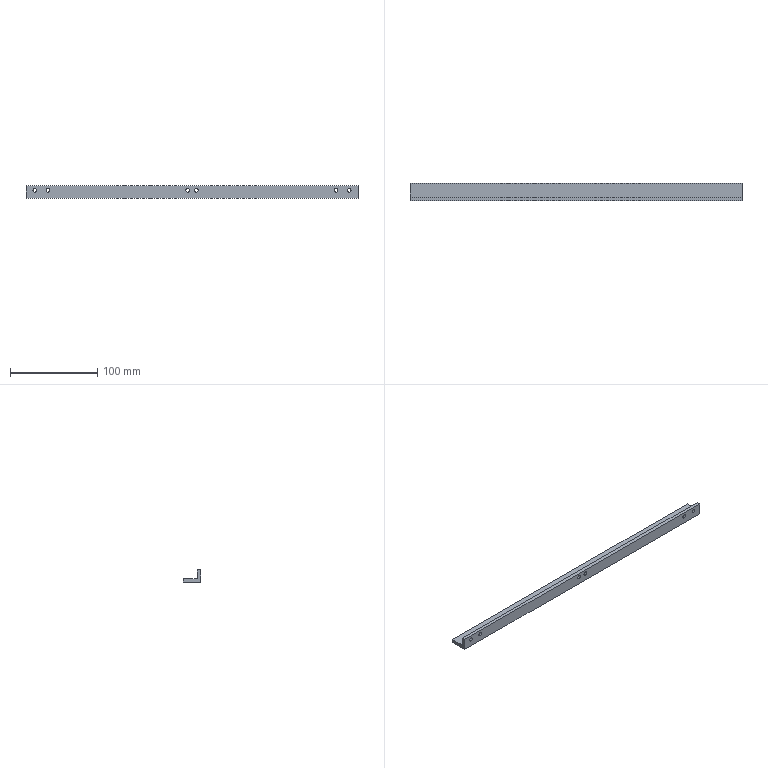Part | SolidWorks | features Extrusion 1, ICE 1 | 1 solid | 20 faces | box 380 x 20 x 14 mm | volume 45267 mm3 | cylinder 12 | plane 8 | commonest cylinder face diameters 4.2 x12
STEP:
#1=CARTESIAN_POINT('',(-5.,4.,-2.1));
#2=VERTEX_POINT('',#1);
#3=CARTESIAN_POINT('',(-5.,4.,2.1));
#4=VERTEX_POINT('',#3);
#5=CARTESIAN_POINT('',(-5.,4.,0.));
#6=DIRECTION('',(0.,1.,0.));
#7=DIRECTION('',(0.,0.,1.));
#8=AXIS2_PLACEMENT_3D('',#5,#6,#7);
#9=CIRCLE('',#8,2.1);
#10=EDGE_CURVE('',#2,#4,#9,.T.);
#11=ORIENTED_EDGE('',*,*,#10,.T.);
#12=CARTESIAN_POINT('',(-5.,0.,2.1));
#13=VERTEX_POINT('',#12);
#14=CARTESIAN_POINT('',(-5.,4.,2.1));
#15=DIRECTION('',(0.,-1.,0.));
#16=VECTOR('',#15,1000.);
#17=LINE('',#14,#16);
#18=EDGE_CURVE('',#4,#13,#17,.T.);
#19=ORIENTED_EDGE('',*,*,#18,.T.);
#20=CARTESIAN_POINT('',(-5.,0.,-2.1));
#21=VERTEX_POINT('',#20);
#22=CARTESIAN_POINT('',(-5.,0.,0.));
#23=DIRECTION('',(0.,1.,0.));
#24=DIRECTION('',(0.,0.,1.));
#25=AXIS2_PLACEMENT_3D('',#22,#23,#24);
#26=CIRCLE('',#25,2.1);
#27=EDGE_CURVE('',#21,#13,#26,.T.);
#28=ORIENTED_EDGE('',*,*,#27,.F.);
#29=CARTESIAN_POINT('',(-5.,4.,-2.1));
#30=DIRECTION('',(0.,-1.,0.));
#31=VECTOR('',#30,1000.);
#32=LINE('',#29,#31);
#33=EDGE_CURVE('',#2,#21,#32,.T.);
#34=ORIENTED_EDGE('',*,*,#33,.F.);
#35=EDGE_LOOP('',(#11,#19,#28,#34));
#36=FACE_OUTER_BOUND('',#35,.T.);
#37=CARTESIAN_POINT('',(-5.,4.,0.));
#38=DIRECTION('',(0.,-1.,0.));
#39=DIRECTION('',(0.,0.,-1.));
#40=AXIS2_PLACEMENT_3D('',#37,#38,#39);
#41=CYLINDRICAL_SURFACE('',#40,2.1);
#42=ADVANCED_FACE('',(#36),#41,.F.);
#43=CARTESIAN_POINT('',(5.,4.,-2.1));
#44=VERTEX_POINT('',#43);
#45=CARTESIAN_POINT('',(5.,4.,2.1));
#46=VERTEX_POINT('',#45);
#47=CARTESIAN_POINT('',(5.,4.,0.));
#48=DIRECTION('',(0.,1.,0.));
#49=DIRECTION('',(0.,0.,1.));
#50=AXIS2_PLACEMENT_3D('',#47,#48,#49);
#51=CIRCLE('',#50,2.1);
#52=EDGE_CURVE('',#44,#46,#51,.T.);
#53=ORIENTED_EDGE('',*,*,#52,.T.);
#54=CARTESIAN_POINT('',(5.,0.,2.1));
#55=VERTEX_POINT('',#54);
#56=CARTESIAN_POINT('',(5.,4.,2.1));
#57=DIRECTION('',(0.,-1.,0.));
#58=VECTOR('',#57,1000.);
#59=LINE('',#56,#58);
#60=EDGE_CURVE('',#46,#55,#59,.T.);
#61=ORIENTED_EDGE('',*,*,#60,.T.);
#62=CARTESIAN_POINT('',(5.,0.,-2.1));
#63=VERTEX_POINT('',#62);
#64=CARTESIAN_POINT('',(5.,0.,0.));
#65=DIRECTION('',(0.,1.,0.));
#66=DIRECTION('',(0.,0.,1.));
#67=AXIS2_PLACEMENT_3D('',#64,#65,#66);
#68=CIRCLE('',#67,2.1);
#69=EDGE_CURVE('',#63,#55,#68,.T.);
#70=ORIENTED_EDGE('',*,*,#69,.F.);
#71=CARTESIAN_POINT('',(5.,4.,-2.1));
#72=DIRECTION('',(0.,-1.,0.));
#73=VECTOR('',#72,1000.);
#74=LINE('',#71,#73);
#75=EDGE_CURVE('',#44,#63,#74,.T.);
#76=ORIENTED_EDGE('',*,*,#75,.F.);
#77=EDGE_LOOP('',(#53,#61,#70,#76));
#78=FACE_OUTER_BOUND('',#77,.T.);
#79=CARTESIAN_POINT('',(5.,4.,0.));
#80=DIRECTION('',(0.,-1.,0.));
#81=DIRECTION('',(0.,0.,-1.));
#82=AXIS2_PLACEMENT_3D('',#79,#80,#81);
#83=CYLINDRICAL_SURFACE('',#82,2.1);
#84=ADVANCED_FACE('',(#78),#83,.F.);
#85=CARTESIAN_POINT('',(180.,4.,-2.1));
#86=VERTEX_POINT('',#85);
#87=CARTESIAN_POINT('',(180.,4.,2.1));
#88=VERTEX_POINT('',#87);
#89=CARTESIAN_POINT('',(180.,4.,0.));
#90=DIRECTION('',(0.,1.,0.));
#91=DIRECTION('',(0.,0.,-1.));
#92=AXIS2_PLACEMENT_3D('',#89,#90,#91);
#93=CIRCLE('',#92,2.1);
#94=EDGE_CURVE('',#86,#88,#93,.T.);
#95=ORIENTED_EDGE('',*,*,#94,.T.);
#96=CARTESIAN_POINT('',(180.,0.,2.1));
#97=VERTEX_POINT('',#96);
#98=CARTESIAN_POINT('',(180.,4.,2.1));
#99=DIRECTION('',(0.,-1.,0.));
#100=VECTOR('',#99,1000.);
#101=LINE('',#98,#100);
#102=EDGE_CURVE('',#88,#97,#101,.T.);
#103=ORIENTED_EDGE('',*,*,#102,.T.);
#104=CARTESIAN_POINT('',(180.,0.,-2.1));
#105=VERTEX_POINT('',#104);
#106=CARTESIAN_POINT('',(180.,0.,0.));
#107=DIRECTION('',(0.,1.,0.));
#108=DIRECTION('',(0.,0.,-1.));
#109=AXIS2_PLACEMENT_3D('',#106,#107,#108);
#110=CIRCLE('',#109,2.1);
#111=EDGE_CURVE('',#105,#97,#110,.T.);
#112=ORIENTED_EDGE('',*,*,#111,.F.);
#113=CARTESIAN_POINT('',(180.,4.,-2.1));
#114=DIRECTION('',(0.,-1.,0.));
#115=VECTOR('',#114,1000.);
#116=LINE('',#113,#115);
#117=EDGE_CURVE('',#86,#105,#116,.T.);
#118=ORIENTED_EDGE('',*,*,#117,.F.);
#119=EDGE_LOOP('',(#95,#103,#112,#118));
#120=FACE_OUTER_BOUND('',#119,.T.);
#121=CARTESIAN_POINT('',(180.,4.,0.));
#122=DIRECTION('',(0.,-1.,0.));
#123=DIRECTION('',(0.,0.,-1.));
#124=AXIS2_PLACEMENT_3D('',#121,#122,#123);
#125=CYLINDRICAL_SURFACE('',#124,2.1);
#126=ADVANCED_FACE('',(#120),#125,.F.);
#127=CARTESIAN_POINT('',(165.,4.,-2.1));
#128=VERTEX_POINT('',#127);
#129=CARTESIAN_POINT('',(165.,4.,2.1));
#130=VERTEX_POINT('',#129);
#131=CARTESIAN_POINT('',(165.,4.,0.));
#132=DIRECTION('',(0.,1.,0.));
#133=DIRECTION('',(0.,0.,-1.));
#134=AXIS2_PLACEMENT_3D('',#131,#132,#133);
#135=CIRCLE('',#134,2.1);
#136=EDGE_CURVE('',#128,#130,#135,.T.);
#137=ORIENTED_EDGE('',*,*,#136,.T.);
#138=CARTESIAN_POINT('',(165.,0.,2.1));
#139=VERTEX_POINT('',#138);
#140=CARTESIAN_POINT('',(165.,4.,2.1));
#141=DIRECTION('',(0.,-1.,0.));
#142=VECTOR('',#141,1000.);
#143=LINE('',#140,#142);
#144=EDGE_CURVE('',#130,#139,#143,.T.);
#145=ORIENTED_EDGE('',*,*,#144,.T.);
#146=CARTESIAN_POINT('',(165.,0.,-2.1));
#147=VERTEX_POINT('',#146);
#148=CARTESIAN_POINT('',(165.,0.,0.));
#149=DIRECTION('',(0.,1.,0.));
#150=DIRECTION('',(0.,0.,-1.));
#151=AXIS2_PLACEMENT_3D('',#148,#149,#150);
#152=CIRCLE('',#151,2.1);
#153=EDGE_CURVE('',#147,#139,#152,.T.);
#154=ORIENTED_EDGE('',*,*,#153,.F.);
#155=CARTESIAN_POINT('',(165.,4.,-2.1));
#156=DIRECTION('',(0.,-1.,0.));
#157=VECTOR('',#156,1000.);
#158=LINE('',#155,#157);
#159=EDGE_CURVE('',#128,#147,#158,.T.);
#160=ORIENTED_EDGE('',*,*,#159,.F.);
#161=EDGE_LOOP('',(#137,#145,#154,#160));
#162=FACE_OUTER_BOUND('',#161,.T.);
#163=CARTESIAN_POINT('',(165.,4.,0.));
#164=DIRECTION('',(0.,-1.,0.));
#165=DIRECTION('',(0.,0.,-1.));
#166=AXIS2_PLACEMENT_3D('',#163,#164,#165);
#167=CYLINDRICAL_SURFACE('',#166,2.1);
#168=ADVANCED_FACE('',(#162),#167,.F.);
#169=CARTESIAN_POINT('',(-165.,4.,-2.1));
#170=VERTEX_POINT('',#169);
#171=CARTESIAN_POINT('',(-165.,4.,2.1));
#172=VERTEX_POINT('',#171);
#173=CARTESIAN_POINT('',(-165.,4.,0.));
#174=DIRECTION('',(0.,1.,0.));
#175=DIRECTION('',(0.,0.,1.));
#176=AXIS2_PLACEMENT_3D('',#173,#174,#175);
#177=CIRCLE('',#176,2.1);
#178=EDGE_CURVE('',#170,#172,#177,.T.);
#179=ORIENTED_EDGE('',*,*,#178,.T.);
#180=CARTESIAN_POINT('',(-165.,0.,2.1));
#181=VERTEX_POINT('',#180);
#182=CARTESIAN_POINT('',(-165.,4.,2.1));
#183=DIRECTION('',(0.,-1.,0.));
#184=VECTOR('',#183,1000.);
#185=LINE('',#182,#184);
#186=EDGE_CURVE('',#172,#181,#185,.T.);
#187=ORIENTED_EDGE('',*,*,#186,.T.);
#188=CARTESIAN_POINT('',(-165.,0.,-2.1));
#189=VERTEX_POINT('',#188);
#190=CARTESIAN_POINT('',(-165.,0.,0.));
#191=DIRECTION('',(0.,1.,0.));
#192=DIRECTION('',(0.,0.,1.));
#193=AXIS2_PLACEMENT_3D('',#190,#191,#192);
#194=CIRCLE('',#193,2.1);
#195=EDGE_CURVE('',#189,#181,#194,.T.);
#196=ORIENTED_EDGE('',*,*,#195,.F.);
#197=CARTESIAN_POINT('',(-165.,4.,-2.1));
#198=DIRECTION('',(0.,-1.,0.));
#199=VECTOR('',#198,1000.);
#200=LINE('',#197,#199);
#201=EDGE_CURVE('',#170,#189,#200,.T.);
#202=ORIENTED_EDGE('',*,*,#201,.F.);
#203=EDGE_LOOP('',(#179,#187,#196,#202));
#204=FACE_OUTER_BOUND('',#203,.T.);
#205=CARTESIAN_POINT('',(-165.,4.,0.));
#206=DIRECTION('',(0.,-1.,0.));
#207=DIRECTION('',(0.,0.,-1.));
#208=AXIS2_PLACEMENT_3D('',#205,#206,#207);
#209=CYLINDRICAL_SURFACE('',#208,2.1);
#210=ADVANCED_FACE('',(#204),#209,.F.);
#211=CARTESIAN_POINT('',(-180.,4.,-2.1));
#212=VERTEX_POINT('',#211);
#213=CARTESIAN_POINT('',(-180.,4.,2.1));
#214=VERTEX_POINT('',#213);
#215=CARTESIAN_POINT('',(-180.,4.,0.));
#216=DIRECTION('',(0.,1.,0.));
#217=DIRECTION('',(0.,0.,1.));
#218=AXIS2_PLACEMENT_3D('',#215,#216,#217);
#219=CIRCLE('',#218,2.1);
#220=EDGE_CURVE('',#212,#214,#219,.T.);
#221=ORIENTED_EDGE('',*,*,#220,.T.);
#222=CARTESIAN_POINT('',(-180.,0.,2.1));
#223=VERTEX_POINT('',#222);
#224=CARTESIAN_POINT('',(-180.,4.,2.1));
#225=DIRECTION('',(0.,-1.,0.));
#226=VECTOR('',#225,1000.);
#227=LINE('',#224,#226);
#228=EDGE_CURVE('',#214,#223,#227,.T.);
#229=ORIENTED_EDGE('',*,*,#228,.T.);
#230=CARTESIAN_POINT('',(-180.,0.,-2.1));
#231=VERTEX_POINT('',#230);
#232=CARTESIAN_POINT('',(-180.,0.,0.));
#233=DIRECTION('',(0.,1.,0.));
#234=DIRECTION('',(0.,0.,1.));
#235=AXIS2_PLACEMENT_3D('',#232,#233,#234);
#236=CIRCLE('',#235,2.1);
#237=EDGE_CURVE('',#231,#223,#236,.T.);
#238=ORIENTED_EDGE('',*,*,#237,.F.);
#239=CARTESIAN_POINT('',(-180.,4.,-2.1));
#240=DIRECTION('',(0.,-1.,0.));
#241=VECTOR('',#240,1000.);
#242=LINE('',#239,#241);
#243=EDGE_CURVE('',#212,#231,#242,.T.);
#244=ORIENTED_EDGE('',*,*,#243,.F.);
#245=EDGE_LOOP('',(#221,#229,#238,#244));
#246=FACE_OUTER_BOUND('',#245,.T.);
#247=CARTESIAN_POINT('',(-180.,4.,0.));
#248=DIRECTION('',(0.,-1.,0.));
#249=DIRECTION('',(0.,0.,-1.));
#250=AXIS2_PLACEMENT_3D('',#247,#248,#249);
#251=CYLINDRICAL_SURFACE('',#250,2.1);
#252=ADVANCED_FACE('',(#246),#251,.F.);
#253=CARTESIAN_POINT('',(190.,4.,5.));
#254=VERTEX_POINT('',#253);
#255=CARTESIAN_POINT('',(190.,4.,-5.));
#256=VERTEX_POINT('',#255);
#257=CARTESIAN_POINT('',(190.,4.,5.));
#258=DIRECTION('',(0.,0.,-1.));
#259=VECTOR('',#258,1000.);
#260=LINE('',#257,#259);
#261=EDGE_CURVE('',#254,#256,#260,.T.);
#262=ORIENTED_EDGE('',*,*,#261,.T.);
#263=CARTESIAN_POINT('',(-190.,4.,-5.));
#264=VERTEX_POINT('',#263);
#265=CARTESIAN_POINT('',(-190.,4.,-5.));
#266=DIRECTION('',(-1.,0.,0.));
#267=VECTOR('',#266,1000.);
#268=LINE('',#265,#267);
#269=EDGE_CURVE('',#256,#264,#268,.T.);
#270=ORIENTED_EDGE('',*,*,#269,.T.);
#271=CARTESIAN_POINT('',(-190.,4.,5.));
#272=VERTEX_POINT('',#271);
#273=CARTESIAN_POINT('',(-190.,4.,5.));
#274=DIRECTION('',(0.,0.,1.));
#275=VECTOR('',#274,1000.);
#276=LINE('',#273,#275);
#277=EDGE_CURVE('',#264,#272,#276,.T.);
#278=ORIENTED_EDGE('',*,*,#277,.T.);
#279=CARTESIAN_POINT('',(-190.,4.,5.));
#280=DIRECTION('',(1.,0.,0.));
#281=VECTOR('',#280,1000.);
#282=LINE('',#279,#281);
#283=EDGE_CURVE('',#272,#254,#282,.T.);
#284=ORIENTED_EDGE('',*,*,#283,.T.);
#285=EDGE_LOOP('',(#262,#270,#278,#284));
#286=FACE_OUTER_BOUND('',#285,.T.);
#287=ORIENTED_EDGE('',*,*,#220,.F.);
#288=CARTESIAN_POINT('',(-180.,4.,0.));
#289=DIRECTION('',(0.,1.,0.));
#290=DIRECTION('',(0.,0.,1.));
#291=AXIS2_PLACEMENT_3D('',#288,#289,#290);
#292=CIRCLE('',#291,2.1);
#293=EDGE_CURVE('',#214,#212,#292,.T.);
#294=ORIENTED_EDGE('',*,*,#293,.F.);
#295=EDGE_LOOP('',(#287,#294));
#296=FACE_BOUND('',#295,.T.);
#297=ORIENTED_EDGE('',*,*,#178,.F.);
#298=CARTESIAN_POINT('',(-165.,4.,0.));
#299=DIRECTION('',(0.,1.,0.));
#300=DIRECTION('',(0.,0.,1.));
#301=AXIS2_PLACEMENT_3D('',#298,#299,#300);
#302=CIRCLE('',#301,2.1);
#303=EDGE_CURVE('',#172,#170,#302,.T.);
#304=ORIENTED_EDGE('',*,*,#303,.F.);
#305=EDGE_LOOP('',(#297,#304));
#306=FACE_BOUND('',#305,.T.);
#307=ORIENTED_EDGE('',*,*,#136,.F.);
#308=CARTESIAN_POINT('',(165.,4.,0.));
#309=DIRECTION('',(0.,1.,0.));
#310=DIRECTION('',(0.,0.,-1.));
#311=AXIS2_PLACEMENT_3D('',#308,#309,#310);
#312=CIRCLE('',#311,2.1);
#313=EDGE_CURVE('',#130,#128,#312,.T.);
#314=ORIENTED_EDGE('',*,*,#313,.F.);
#315=EDGE_LOOP('',(#307,#314));
#316=FACE_BOUND('',#315,.T.);
#317=ORIENTED_EDGE('',*,*,#94,.F.);
#318=CARTESIAN_POINT('',(180.,4.,0.));
#319=DIRECTION('',(0.,1.,0.));
#320=DIRECTION('',(0.,0.,-1.));
#321=AXIS2_PLACEMENT_3D('',#318,#319,#320);
#322=CIRCLE('',#321,2.1);
#323=EDGE_CURVE('',#88,#86,#322,.T.);
#324=ORIENTED_EDGE('',*,*,#323,.F.);
#325=EDGE_LOOP('',(#317,#324));
#326=FACE_BOUND('',#325,.T.);
#327=ORIENTED_EDGE('',*,*,#52,.F.);
#328=CARTESIAN_POINT('',(5.,4.,0.));
#329=DIRECTION('',(0.,1.,0.));
#330=DIRECTION('',(0.,0.,1.));
#331=AXIS2_PLACEMENT_3D('',#328,#329,#330);
#332=CIRCLE('',#331,2.1);
#333=EDGE_CURVE('',#46,#44,#332,.T.);
#334=ORIENTED_EDGE('',*,*,#333,.F.);
#335=EDGE_LOOP('',(#327,#334));
#336=FACE_BOUND('',#335,.T.);
#337=ORIENTED_EDGE('',*,*,#10,.F.);
#338=CARTESIAN_POINT('',(-5.,4.,0.));
#339=DIRECTION('',(0.,1.,0.));
#340=DIRECTION('',(0.,0.,1.));
#341=AXIS2_PLACEMENT_3D('',#338,#339,#340);
#342=CIRCLE('',#341,2.1);
#343=EDGE_CURVE('',#4,#2,#342,.T.);
#344=ORIENTED_EDGE('',*,*,#343,.F.);
#345=EDGE_LOOP('',(#337,#344));
#346=FACE_BOUND('',#345,.T.);
#347=CARTESIAN_POINT('',(0.,4.,0.));
#348=DIRECTION('',(0.,-1.,0.));
#349=DIRECTION('',(0.,0.,-1.));
#350=AXIS2_PLACEMENT_3D('',#347,#348,#349);
#351=PLANE('',#350);
#352=ADVANCED_FACE('',(#286,#296,#306,#316,#326,#336,#346),#351,.F.);
#353=ORIENTED_EDGE('',*,*,#69,.T.);
#354=CARTESIAN_POINT('',(5.,0.,0.));
#355=DIRECTION('',(0.,1.,0.));
#356=DIRECTION('',(0.,0.,1.));
#357=AXIS2_PLACEMENT_3D('',#354,#355,#356);
#358=CIRCLE('',#357,2.1);
#359=EDGE_CURVE('',#55,#63,#358,.T.);
#360=ORIENTED_EDGE('',*,*,#359,.T.);
#361=EDGE_LOOP('',(#353,#360));
#362=FACE_BOUND('',#361,.T.);
#363=ORIENTED_EDGE('',*,*,#153,.T.);
#364=CARTESIAN_POINT('',(165.,0.,0.));
#365=DIRECTION('',(0.,1.,0.));
#366=DIRECTION('',(0.,0.,-1.));
#367=AXIS2_PLACEMENT_3D('',#364,#365,#366);
#368=CIRCLE('',#367,2.1);
#369=EDGE_CURVE('',#139,#147,#368,.T.);
#370=ORIENTED_EDGE('',*,*,#369,.T.);
#371=EDGE_LOOP('',(#363,#370));
#372=FACE_BOUND('',#371,.T.);
#373=ORIENTED_EDGE('',*,*,#237,.T.);
#374=CARTESIAN_POINT('',(-180.,0.,0.));
#375=DIRECTION('',(0.,1.,0.));
#376=DIRECTION('',(0.,0.,1.));
#377=AXIS2_PLACEMENT_3D('',#374,#375,#376);
#378=CIRCLE('',#377,2.1);
#379=EDGE_CURVE('',#223,#231,#378,.T.);
#380=ORIENTED_EDGE('',*,*,#379,.T.);
#381=EDGE_LOOP('',(#373,#380));
#382=FACE_BOUND('',#381,.T.);
#383=CARTESIAN_POINT('',(190.,0.,5.));
#384=VERTEX_POINT('',#383);
#385=CARTESIAN_POINT('',(190.,0.,-9.));
#386=VERTEX_POINT('',#385);
#387=CARTESIAN_POINT('',(190.,0.,5.));
#388=DIRECTION('',(0.,0.,-1.));
#389=VECTOR('',#388,1000.);
#390=LINE('',#387,#389);
#391=EDGE_CURVE('',#384,#386,#390,.T.);
#392=ORIENTED_EDGE('',*,*,#391,.F.);
#393=CARTESIAN_POINT('',(-190.,0.,5.));
#394=VERTEX_POINT('',#393);
#395=CARTESIAN_POINT('',(-190.,0.,5.));
#396=DIRECTION('',(1.,0.,0.));
#397=VECTOR('',#396,1000.);
#398=LINE('',#395,#397);
#399=EDGE_CURVE('',#394,#384,#398,.T.);
#400=ORIENTED_EDGE('',*,*,#399,.F.);
#401=CARTESIAN_POINT('',(-190.,0.,-9.));
#402=VERTEX_POINT('',#401);
#403=CARTESIAN_POINT('',(-190.,0.,5.));
#404=DIRECTION('',(0.,0.,1.));
#405=VECTOR('',#404,1000.);
#406=LINE('',#403,#405);
#407=EDGE_CURVE('',#402,#394,#406,.T.);
#408=ORIENTED_EDGE('',*,*,#407,.F.);
#409=CARTESIAN_POINT('',(190.,0.,-9.));
#410=DIRECTION('',(-1.,0.,0.));
#411=VECTOR('',#410,1000.);
#412=LINE('',#409,#411);
#413=EDGE_CURVE('',#386,#402,#412,.T.);
#414=ORIENTED_EDGE('',*,*,#413,.F.);
#415=EDGE_LOOP('',(#392,#400,#408,#414));
#416=FACE_OUTER_BOUND('',#415,.T.);
#417=ORIENTED_EDGE('',*,*,#195,.T.);
#418=CARTESIAN_POINT('',(-165.,0.,0.));
#419=DIRECTION('',(0.,1.,0.));
#420=DIRECTION('',(0.,0.,1.));
#421=AXIS2_PLACEMENT_3D('',#418,#419,#420);
#422=CIRCLE('',#421,2.1);
#423=EDGE_CURVE('',#181,#189,#422,.T.);
#424=ORIENTED_EDGE('',*,*,#423,.T.);
#425=EDGE_LOOP('',(#417,#424));
#426=FACE_BOUND('',#425,.T.);
#427=ORIENTED_EDGE('',*,*,#111,.T.);
#428=CARTESIAN_POINT('',(180.,0.,0.));
#429=DIRECTION('',(0.,1.,0.));
#430=DIRECTION('',(0.,0.,-1.));
#431=AXIS2_PLACEMENT_3D('',#428,#429,#430);
#432=CIRCLE('',#431,2.1);
#433=EDGE_CURVE('',#97,#105,#432,.T.);
#434=ORIENTED_EDGE('',*,*,#433,.T.);
#435=EDGE_LOOP('',(#427,#434));
#436=FACE_BOUND('',#435,.T.);
#437=ORIENTED_EDGE('',*,*,#27,.T.);
#438=CARTESIAN_POINT('',(-5.,0.,0.));
#439=DIRECTION('',(0.,1.,0.));
#440=DIRECTION('',(0.,0.,1.));
#441=AXIS2_PLACEMENT_3D('',#438,#439,#440);
#442=CIRCLE('',#441,2.1);
#443=EDGE_CURVE('',#13,#21,#442,.T.);
#444=ORIENTED_EDGE('',*,*,#443,.T.);
#445=EDGE_LOOP('',(#437,#444));
#446=FACE_BOUND('',#445,.T.);
#447=CARTESIAN_POINT('',(0.,0.,0.));
#448=DIRECTION('',(0.,-1.,0.));
#449=DIRECTION('',(0.,0.,-1.));
#450=AXIS2_PLACEMENT_3D('',#447,#448,#449);
#451=PLANE('',#450);
#452=ADVANCED_FACE('',(#362,#372,#382,#416,#426,#436,#446),#451,.T.);
#453=ORIENTED_EDGE('',*,*,#391,.T.);
#454=CARTESIAN_POINT('',(190.,20.,-9.));
#455=VERTEX_POINT('',#454);
#456=CARTESIAN_POINT('',(190.,0.,-9.));
#457=DIRECTION('',(0.,-1.,0.));
#458=VECTOR('',#457,1000.);
#459=LINE('',#456,#458);
#460=EDGE_CURVE('',#455,#386,#459,.T.);
#461=ORIENTED_EDGE('',*,*,#460,.F.);
#462=CARTESIAN_POINT('',(190.,20.,-5.));
#463=VERTEX_POINT('',#462);
#464=CARTESIAN_POINT('',(190.,20.,-9.));
#465=DIRECTION('',(0.,0.,1.));
#466=VECTOR('',#465,1000.);
#467=LINE('',#464,#466);
#468=EDGE_CURVE('',#455,#463,#467,.T.);
#469=ORIENTED_EDGE('',*,*,#468,.T.);
#470=CARTESIAN_POINT('',(190.,0.,-5.));
#471=DIRECTION('',(0.,-1.,0.));
#472=VECTOR('',#471,1000.);
#473=LINE('',#470,#472);
#474=EDGE_CURVE('',#463,#256,#473,.T.);
#475=ORIENTED_EDGE('',*,*,#474,.T.);
#476=ORIENTED_EDGE('',*,*,#261,.F.);
#477=CARTESIAN_POINT('',(190.,4.,5.));
#478=DIRECTION('',(0.,-1.,0.));
#479=VECTOR('',#478,1000.);
#480=LINE('',#477,#479);
#481=EDGE_CURVE('',#254,#384,#480,.T.);
#482=ORIENTED_EDGE('',*,*,#481,.T.);
#483=EDGE_LOOP('',(#453,#461,#469,#475,#476,#482));
#484=FACE_OUTER_BOUND('',#483,.T.);
#485=CARTESIAN_POINT('',(190.,4.,5.));
#486=DIRECTION('',(-1.,0.,0.));
#487=DIRECTION('',(0.,0.,1.));
#488=AXIS2_PLACEMENT_3D('',#485,#486,#487);
#489=PLANE('',#488);
#490=ADVANCED_FACE('',(#484),#489,.F.);
#491=ORIENTED_EDGE('',*,*,#407,.T.);
#492=CARTESIAN_POINT('',(-190.,4.,5.));
#493=DIRECTION('',(0.,-1.,0.));
#494=VECTOR('',#493,1000.);
#495=LINE('',#492,#494);
#496=EDGE_CURVE('',#272,#394,#495,.T.);
#497=ORIENTED_EDGE('',*,*,#496,.F.);
#498=ORIENTED_EDGE('',*,*,#277,.F.);
#499=CARTESIAN_POINT('',(-190.,20.,-5.));
#500=VERTEX_POINT('',#499);
#501=CARTESIAN_POINT('',(-190.,0.,-5.));
#502=DIRECTION('',(0.,1.,0.));
#503=VECTOR('',#502,1000.);
#504=LINE('',#501,#503);
#505=EDGE_CURVE('',#264,#500,#504,.T.);
#506=ORIENTED_EDGE('',*,*,#505,.T.);
#507=CARTESIAN_POINT('',(-190.,20.,-9.));
#508=VERTEX_POINT('',#507);
#509=CARTESIAN_POINT('',(-190.,20.,-9.));
#510=DIRECTION('',(0.,0.,1.));
#511=VECTOR('',#510,1000.);
#512=LINE('',#509,#511);
#513=EDGE_CURVE('',#508,#500,#512,.T.);
#514=ORIENTED_EDGE('',*,*,#513,.F.);
#515=CARTESIAN_POINT('',(-190.,0.,-9.));
#516=DIRECTION('',(0.,1.,0.));
#517=VECTOR('',#516,1000.);
#518=LINE('',#515,#517);
#519=EDGE_CURVE('',#402,#508,#518,.T.);
#520=ORIENTED_EDGE('',*,*,#519,.F.);
#521=EDGE_LOOP('',(#491,#497,#498,#506,#514,#520));
#522=FACE_OUTER_BOUND('',#521,.T.);
#523=CARTESIAN_POINT('',(-190.,4.,5.));
#524=DIRECTION('',(1.,0.,0.));
#525=DIRECTION('',(0.,0.,-1.));
#526=AXIS2_PLACEMENT_3D('',#523,#524,#525);
#527=PLANE('',#526);
#528=ADVANCED_FACE('',(#522),#527,.F.);
#529=ORIENTED_EDGE('',*,*,#399,.T.);
#530=ORIENTED_EDGE('',*,*,#481,.F.);
#531=ORIENTED_EDGE('',*,*,#283,.F.);
#532=ORIENTED_EDGE('',*,*,#496,.T.);
#533=EDGE_LOOP('',(#529,#530,#531,#532));
#534=FACE_OUTER_BOUND('',#533,.T.);
#535=CARTESIAN_POINT('',(-190.,4.,5.));
#536=DIRECTION('',(0.,0.,-1.));
#537=DIRECTION('',(-1.,0.,0.));
#538=AXIS2_PLACEMENT_3D('',#535,#536,#537);
#539=PLANE('',#538);
#540=ADVANCED_FACE('',(#534),#539,.F.);
#541=ORIENTED_EDGE('',*,*,#228,.F.);
#542=ORIENTED_EDGE('',*,*,#293,.T.);
#543=ORIENTED_EDGE('',*,*,#243,.T.);
#544=ORIENTED_EDGE('',*,*,#379,.F.);
#545=EDGE_LOOP('',(#541,#542,#543,#544));
#546=FACE_OUTER_BOUND('',#545,.T.);
#547=CARTESIAN_POINT('',(-180.,4.,0.));
#548=DIRECTION('',(0.,-1.,0.));
#549=DIRECTION('',(0.,0.,-1.));
#550=AXIS2_PLACEMENT_3D('',#547,#548,#549);
#551=CYLINDRICAL_SURFACE('',#550,2.1);
#552=ADVANCED_FACE('',(#546),#551,.F.);
#553=ORIENTED_EDGE('',*,*,#186,.F.);
#554=ORIENTED_EDGE('',*,*,#303,.T.);
#555=ORIENTED_EDGE('',*,*,#201,.T.);
#556=ORIENTED_EDGE('',*,*,#423,.F.);
#557=EDGE_LOOP('',(#553,#554,#555,#556));
#558=FACE_OUTER_BOUND('',#557,.T.);
#559=CARTESIAN_POINT('',(-165.,4.,0.));
#560=DIRECTION('',(0.,-1.,0.));
#561=DIRECTION('',(0.,0.,-1.));
#562=AXIS2_PLACEMENT_3D('',#559,#560,#561);
#563=CYLINDRICAL_SURFACE('',#562,2.1);
#564=ADVANCED_FACE('',(#558),#563,.F.);
#565=ORIENTED_EDGE('',*,*,#144,.F.);
#566=ORIENTED_EDGE('',*,*,#313,.T.);
#567=ORIENTED_EDGE('',*,*,#159,.T.);
#568=ORIENTED_EDGE('',*,*,#369,.F.);
#569=EDGE_LOOP('',(#565,#566,#567,#568));
#570=FACE_OUTER_BOUND('',#569,.T.);
#571=CARTESIAN_POINT('',(165.,4.,0.));
#572=DIRECTION('',(0.,-1.,0.));
#573=DIRECTION('',(0.,0.,-1.));
#574=AXIS2_PLACEMENT_3D('',#571,#572,#573);
#575=CYLINDRICAL_SURFACE('',#574,2.1);
#576=ADVANCED_FACE('',(#570),#575,.F.);
#577=ORIENTED_EDGE('',*,*,#102,.F.);
#578=ORIENTED_EDGE('',*,*,#323,.T.);
#579=ORIENTED_EDGE('',*,*,#117,.T.);
#580=ORIENTED_EDGE('',*,*,#433,.F.);
#581=EDGE_LOOP('',(#577,#578,#579,#580));
#582=FACE_OUTER_BOUND('',#581,.T.);
#583=CARTESIAN_POINT('',(180.,4.,0.));
#584=DIRECTION('',(0.,-1.,0.));
#585=DIRECTION('',(0.,0.,-1.));
#586=AXIS2_PLACEMENT_3D('',#583,#584,#585);
#587=CYLINDRICAL_SURFACE('',#586,2.1);
#588=ADVANCED_FACE('',(#582),#587,.F.);
#589=ORIENTED_EDGE('',*,*,#60,.F.);
#590=ORIENTED_EDGE('',*,*,#333,.T.);
#591=ORIENTED_EDGE('',*,*,#75,.T.);
#592=ORIENTED_EDGE('',*,*,#359,.F.);
#593=EDGE_LOOP('',(#589,#590,#591,#592));
#594=FACE_OUTER_BOUND('',#593,.T.);
#595=CARTESIAN_POINT('',(5.,4.,0.));
#596=DIRECTION('',(0.,-1.,0.));
#597=DIRECTION('',(0.,0.,-1.));
#598=AXIS2_PLACEMENT_3D('',#595,#596,#597);
#599=CYLINDRICAL_SURFACE('',#598,2.1);
#600=ADVANCED_FACE('',(#594),#599,.F.);
#601=ORIENTED_EDGE('',*,*,#18,.F.);
#602=ORIENTED_EDGE('',*,*,#343,.T.);
#603=ORIENTED_EDGE('',*,*,#33,.T.);
#604=ORIENTED_EDGE('',*,*,#443,.F.);
#605=EDGE_LOOP('',(#601,#602,#603,#604));
#606=FACE_OUTER_BOUND('',#605,.T.);
#607=CARTESIAN_POINT('',(-5.,4.,0.));
#608=DIRECTION('',(0.,-1.,0.));
#609=DIRECTION('',(0.,0.,-1.));
#610=AXIS2_PLACEMENT_3D('',#607,#608,#609);
#611=CYLINDRICAL_SURFACE('',#610,2.1);
#612=ADVANCED_FACE('',(#606),#611,.F.);
#613=ORIENTED_EDGE('',*,*,#269,.F.);
#614=ORIENTED_EDGE('',*,*,#474,.F.);
#615=CARTESIAN_POINT('',(190.,20.,-5.));
#616=DIRECTION('',(1.,0.,0.));
#617=VECTOR('',#616,1000.);
#618=LINE('',#615,#617);
#619=EDGE_CURVE('',#500,#463,#618,.T.);
#620=ORIENTED_EDGE('',*,*,#619,.F.);
#621=ORIENTED_EDGE('',*,*,#505,.F.);
#622=EDGE_LOOP('',(#613,#614,#620,#621));
#623=FACE_OUTER_BOUND('',#622,.T.);
#624=CARTESIAN_POINT('',(0.,0.,-5.));
#625=DIRECTION('',(0.,0.,1.));
#626=DIRECTION('',(1.,0.,0.));
#627=AXIS2_PLACEMENT_3D('',#624,#625,#626);
#628=PLANE('',#627);
#629=ADVANCED_FACE('',(#623),#628,.T.);
#630=ORIENTED_EDGE('',*,*,#619,.T.);
#631=ORIENTED_EDGE('',*,*,#468,.F.);
#632=CARTESIAN_POINT('',(190.,20.,-9.));
#633=DIRECTION('',(1.,0.,0.));
#634=VECTOR('',#633,1000.);
#635=LINE('',#632,#634);
#636=EDGE_CURVE('',#508,#455,#635,.T.);
#637=ORIENTED_EDGE('',*,*,#636,.F.);
#638=ORIENTED_EDGE('',*,*,#513,.T.);
#639=EDGE_LOOP('',(#630,#631,#637,#638));
#640=FACE_OUTER_BOUND('',#639,.T.);
#641=CARTESIAN_POINT('',(190.,20.,-9.));
#642=DIRECTION('',(0.,-1.,0.));
#643=DIRECTION('',(0.,0.,-1.));
#644=AXIS2_PLACEMENT_3D('',#641,#642,#643);
#645=PLANE('',#644);
#646=ADVANCED_FACE('',(#640),#645,.F.);
#647=ORIENTED_EDGE('',*,*,#460,.T.);
#648=ORIENTED_EDGE('',*,*,#413,.T.);
#649=ORIENTED_EDGE('',*,*,#519,.T.);
#650=ORIENTED_EDGE('',*,*,#636,.T.);
#651=EDGE_LOOP('',(#647,#648,#649,#650));
#652=FACE_OUTER_BOUND('',#651,.T.);
#653=CARTESIAN_POINT('',(0.,0.,-9.));
#654=DIRECTION('',(0.,0.,1.));
#655=DIRECTION('',(1.,0.,0.));
#656=AXIS2_PLACEMENT_3D('',#653,#654,#655);
#657=PLANE('',#656);
#658=ADVANCED_FACE('',(#652),#657,.F.);
#659=CLOSED_SHELL('',(#42,#84,#126,#168,#210,#252,#352,#452,#490,#528,#540,#552,#564,#576,#588,#600,#612,#629,#646,#658));
#660=MANIFOLD_SOLID_BREP('',#659);
#661=CARTESIAN_POINT('',(0.,0.,0.));
#662=DIRECTION('',(0.,0.,1.));
#663=DIRECTION('',(1.,0.,0.));
#664=AXIS2_PLACEMENT_3D('',#661,#662,#663);
#665=(LENGTH_UNIT()NAMED_UNIT(*)SI_UNIT(.MILLI.,.METRE.));
#666=UNCERTAINTY_MEASURE_WITH_UNIT(LENGTH_MEASURE(0.00001),#665,'','');
#667=(NAMED_UNIT(*)PLANE_ANGLE_UNIT()SI_UNIT($,.RADIAN.));
#668=(NAMED_UNIT(*)SI_UNIT($,.STERADIAN.)SOLID_ANGLE_UNIT());
#669=(GEOMETRIC_REPRESENTATION_CONTEXT(3)GLOBAL_UNCERTAINTY_ASSIGNED_CONTEXT((#666))GLOBAL_UNIT_ASSIGNED_CONTEXT((#665,#667,#668))REPRESENTATION_CONTEXT('',''));
#670=ADVANCED_BREP_SHAPE_REPRESENTATION('',(#660,#664),#669);